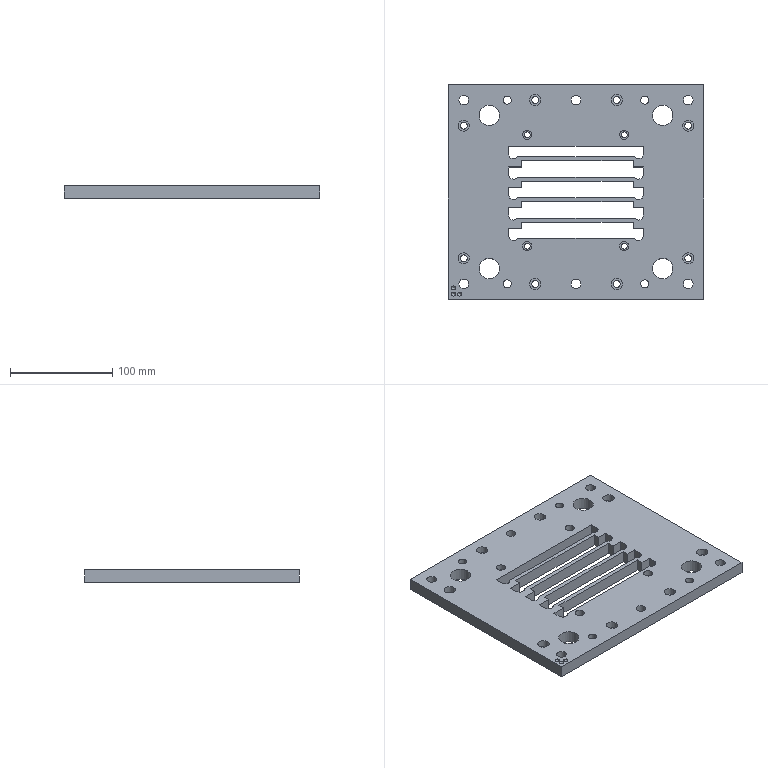Part | STEP file | 200 mesh_id2094 | 1 solid | 105 faces | box 250 x 210 x 12 mm | volume 486087 mm3 | plane 54 | cylinder 48 | cone 3 | commonest cylinder face diameters 10 x10 6.8 x8 11 x8 9.5 x6 5.8 x4 8 x4